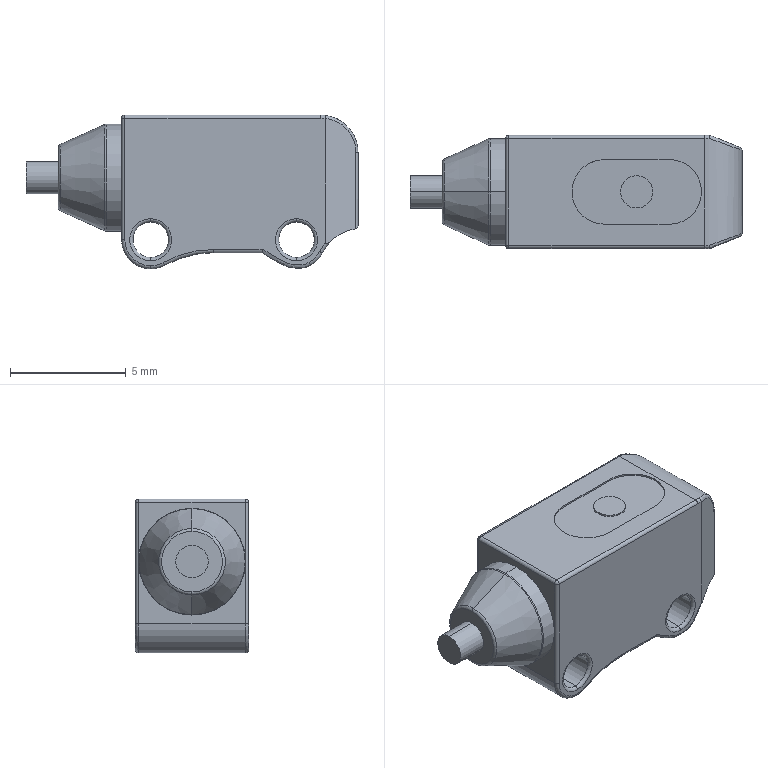Part | SolidWorks | features SplitBody 1 | 1 solid | 76 faces | box 14.35 x 4.9 x 6.65 mm | volume 315.271 mm3 | cylinder 28 | torus 24 | plane 15 | spline 5 | cone 2 | sphere 2 | commonest cylinder face diameters 0.28 x10 1.4 x4 1.54 x4 2.8 x3 4.62 x2 2.52 x1